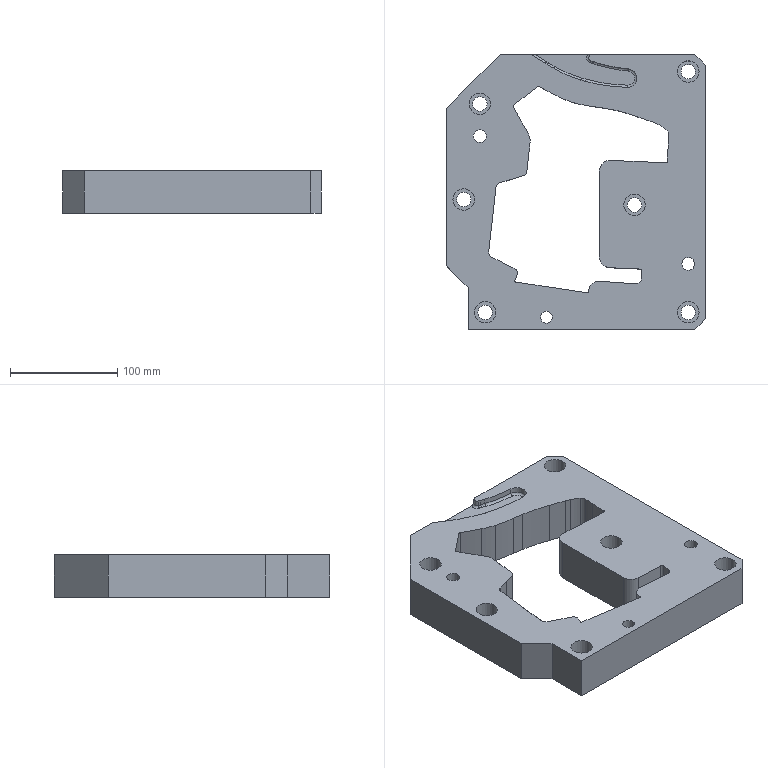Part | NX | features 23 2 | 1 solid | 108 faces | box 241 x 256 x 40 mm | volume 1575451 mm3 | cylinder 47 | plane 38 | spline 19 | torus 4 | commonest cylinder face diameters 20 x8 13.5 x6 2 x5 10 x3 3 x2 12.001 x2